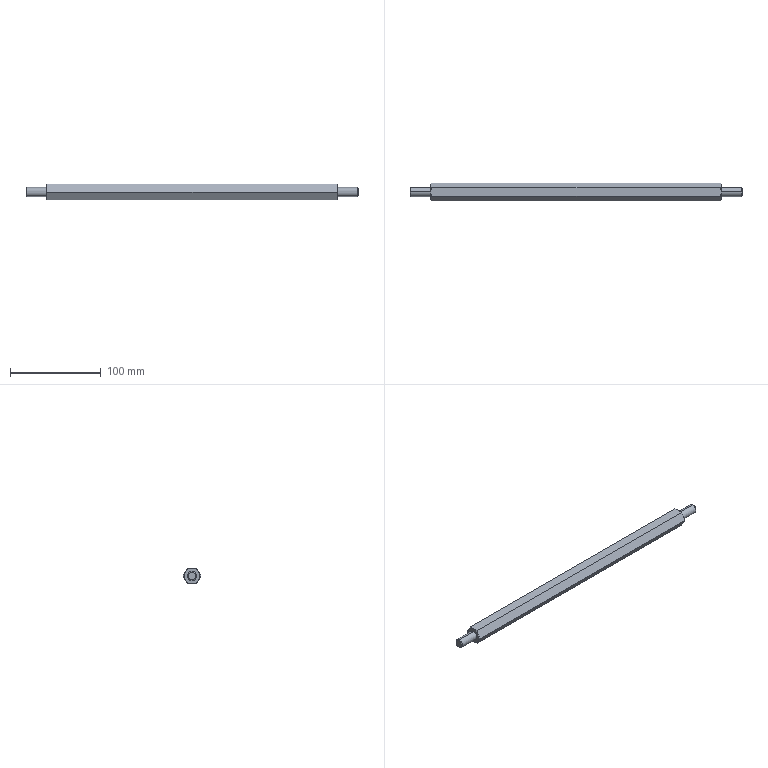Part | STEP file | _PLSBM17-320-M10-N10.stp | 1 solid | 30 faces | box 366 x 19.63 x 17 mm | volume 83661 mm3 | cone 16 | plane 10 | cylinder 4 | commonest cylinder face diameters 10 x4